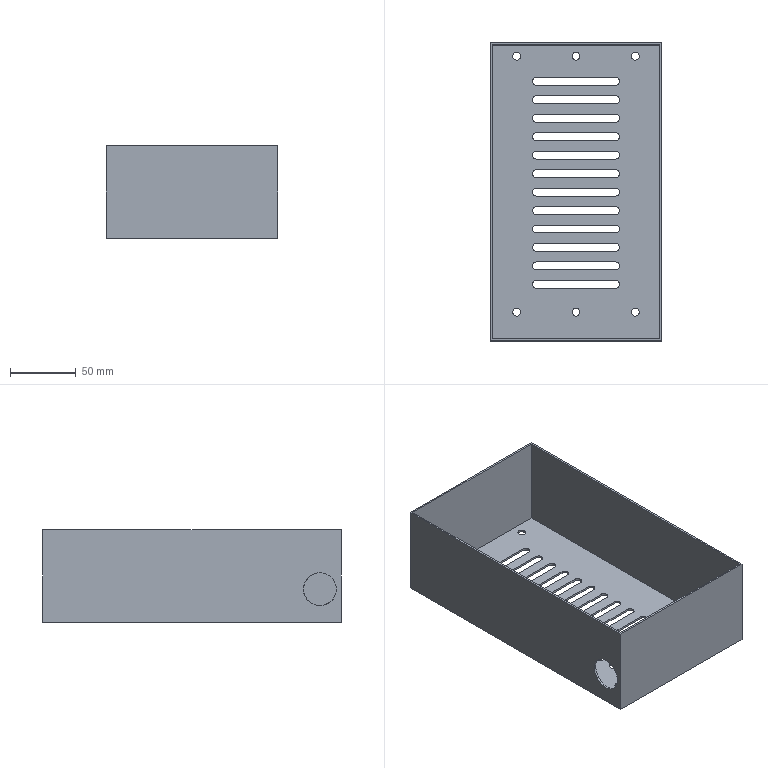Part | NX | features EXTRUDE 3, DATUM_CSYS 2, SKETCH 2, LINKED_FACE 1 | 1 solid | 66 faces | box 130 x 226 x 70 mm | volume 108632 mm3 | plane 35 | cylinder 31 | commonest cylinder face diameters 6 x30 25 x1